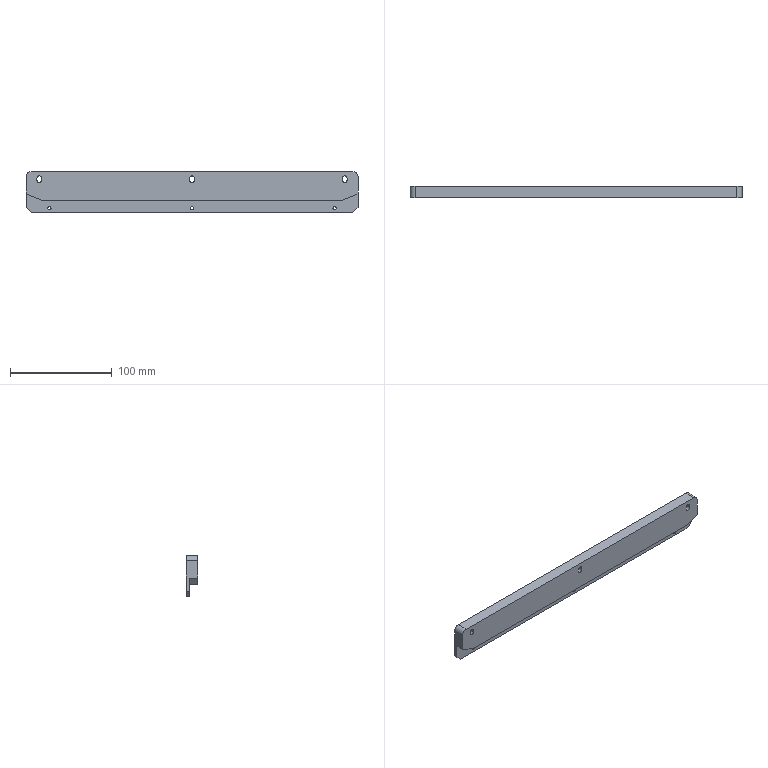Part | STEP file | upper limit plate 1 | 1 solid | 53 faces | box 326 x 11 x 40 mm | volume 109712 mm3 | plane 27 | cylinder 26 | commonest cylinder face diameters 4.5 x9 8 x9 3.3 x6 10 x2